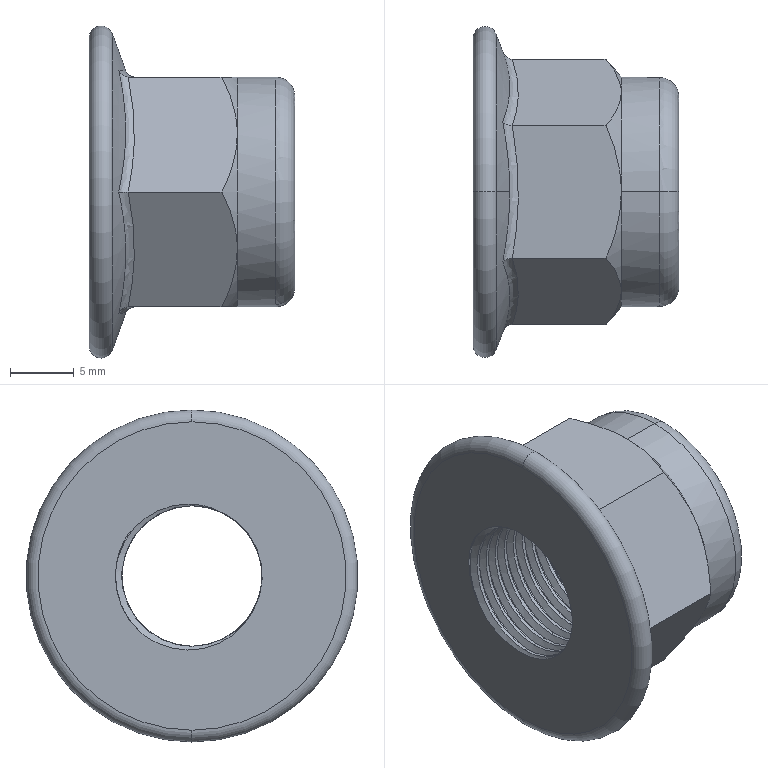Part | STEP file | Torque nut 04-2_ISO(ISO 7043-M12-N)_Valor predeterminado | 1 solid | 95 faces | box 16.1 x 26 x 26 mm | volume 3173 mm3 | cylinder 63 | cone 10 | plane 10 | spline 8 | torus 4 | commonest cylinder face diameters 12 x30 11 x29 13.5 x2 18 x2